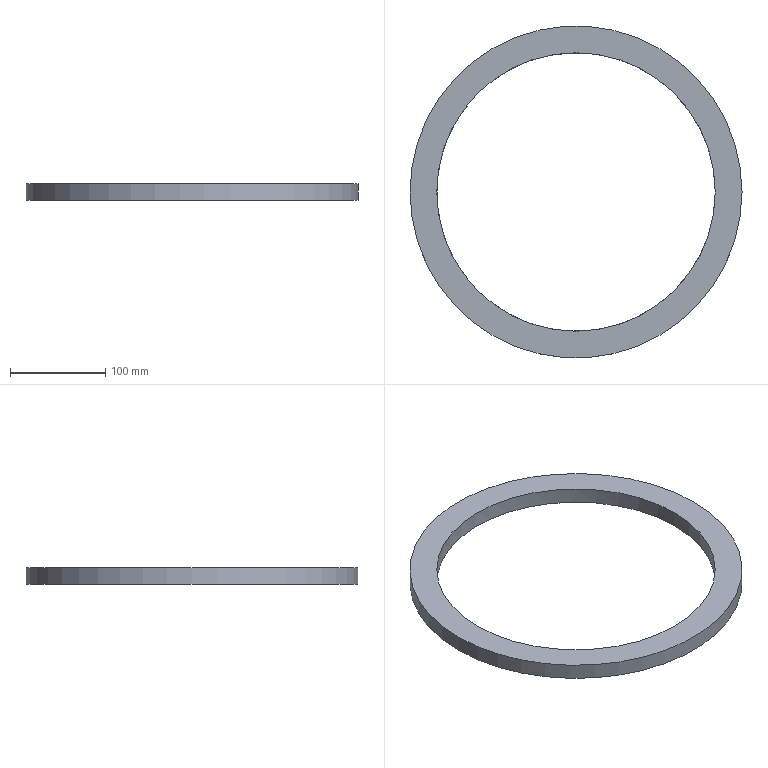Part | NX | features CYLINDER 2, DATUM_CSYS 1, Delete Body 1, LINKED_BODY 1, SCALE 1 | 1 solid | 4 faces | box 348.75 x 348.75 x 16.875 mm | volume 478061 mm3 | plane 2 | cylinder 2 | commonest cylinder face diameters 292.5 x1 348.75 x1
STEP:
#1=CARTESIAN_POINT('',(-512.832,-1724.979,-139.));
#2=VERTEX_POINT('',#1);
#3=CARTESIAN_POINT('',(-366.582,-1724.979,-139.));
#4=DIRECTION('',(0.,0.,-1.));
#5=DIRECTION('',(-1.,0.,0.));
#6=AXIS2_PLACEMENT_3D('',#3,#4,#5);
#7=CIRCLE('',#6,146.25);
#8=EDGE_CURVE('',#2,#2,#7,.T.);
#9=ORIENTED_EDGE('',*,*,#8,.T.);
#10=EDGE_LOOP('',(#9));
#11=FACE_BOUND('',#10,.T.);
#12=CARTESIAN_POINT('',(-540.957,-1724.979,-139.));
#13=VERTEX_POINT('',#12);
#14=CARTESIAN_POINT('',(-366.582,-1724.979,-139.));
#15=DIRECTION('',(0.,0.,-1.));
#16=DIRECTION('',(-1.,0.,0.));
#17=AXIS2_PLACEMENT_3D('',#14,#15,#16);
#18=CIRCLE('',#17,174.375);
#19=EDGE_CURVE('',#13,#13,#18,.T.);
#20=ORIENTED_EDGE('',*,*,#19,.F.);
#21=EDGE_LOOP('',(#20));
#22=FACE_BOUND('',#21,.T.);
#23=CARTESIAN_POINT('',(-366.582,-1724.979,-139.));
#24=DIRECTION('',(0.,0.,1.));
#25=DIRECTION('',(1.,0.,0.));
#26=AXIS2_PLACEMENT_3D('',#23,#24,#25);
#27=PLANE('',#26);
#28=ADVANCED_FACE('',(#11,#22),#27,.T.);
#29=CARTESIAN_POINT('',(-220.332,-1724.979,-155.875));
#30=VERTEX_POINT('',#29);
#31=CARTESIAN_POINT('',(-366.582,-1724.979,-155.875));
#32=DIRECTION('',(0.,0.,1.));
#33=DIRECTION('',(1.,0.,0.));
#34=AXIS2_PLACEMENT_3D('',#31,#32,#33);
#35=CIRCLE('',#34,146.25);
#36=EDGE_CURVE('',#30,#30,#35,.T.);
#37=ORIENTED_EDGE('',*,*,#36,.T.);
#38=EDGE_LOOP('',(#37));
#39=FACE_BOUND('',#38,.T.);
#40=CARTESIAN_POINT('',(-192.207,-1724.979,-155.875));
#41=VERTEX_POINT('',#40);
#42=CARTESIAN_POINT('',(-366.582,-1724.979,-155.875));
#43=DIRECTION('',(0.,0.,1.));
#44=DIRECTION('',(1.,0.,0.));
#45=AXIS2_PLACEMENT_3D('',#42,#43,#44);
#46=CIRCLE('',#45,174.375);
#47=EDGE_CURVE('',#41,#41,#46,.T.);
#48=ORIENTED_EDGE('',*,*,#47,.F.);
#49=EDGE_LOOP('',(#48));
#50=FACE_BOUND('',#49,.T.);
#51=CARTESIAN_POINT('',(-366.582,-1724.979,-155.875));
#52=DIRECTION('',(0.,0.,-1.));
#53=DIRECTION('',(-1.,0.,0.));
#54=AXIS2_PLACEMENT_3D('',#51,#52,#53);
#55=PLANE('',#54);
#56=ADVANCED_FACE('',(#39,#50),#55,.T.);
#57=ORIENTED_EDGE('',*,*,#19,.T.);
#58=EDGE_LOOP('',(#57));
#59=FACE_BOUND('',#58,.T.);
#60=ORIENTED_EDGE('',*,*,#47,.T.);
#61=EDGE_LOOP('',(#60));
#62=FACE_BOUND('',#61,.T.);
#63=CARTESIAN_POINT('',(-366.582,-1724.979,-155.875));
#64=DIRECTION('',(0.,0.,1.));
#65=DIRECTION('',(1.,0.,0.));
#66=AXIS2_PLACEMENT_3D('',#63,#64,#65);
#67=CYLINDRICAL_SURFACE('',#66,174.375);
#68=ADVANCED_FACE('',(#59,#62),#67,.T.);
#69=ORIENTED_EDGE('',*,*,#8,.F.);
#70=EDGE_LOOP('',(#69));
#71=FACE_BOUND('',#70,.T.);
#72=ORIENTED_EDGE('',*,*,#36,.F.);
#73=EDGE_LOOP('',(#72));
#74=FACE_BOUND('',#73,.T.);
#75=CARTESIAN_POINT('',(-366.582,-1724.979,-155.875));
#76=DIRECTION('',(0.,0.,1.));
#77=DIRECTION('',(1.,0.,0.));
#78=AXIS2_PLACEMENT_3D('',#75,#76,#77);
#79=CYLINDRICAL_SURFACE('',#78,146.25);
#80=ADVANCED_FACE('',(#71,#74),#79,.F.);
#81=CLOSED_SHELL('',(#28,#56,#68,#80));
#82=MANIFOLD_SOLID_BREP('',#81);
#83=(LENGTH_UNIT()NAMED_UNIT(*)SI_UNIT(.MILLI.,.METRE.));
#84=UNCERTAINTY_MEASURE_WITH_UNIT(LENGTH_MEASURE(0.00001),#83,'','');
#85=(NAMED_UNIT(*)PLANE_ANGLE_UNIT()SI_UNIT($,.RADIAN.));
#86=(NAMED_UNIT(*)SI_UNIT($,.STERADIAN.)SOLID_ANGLE_UNIT());
#87=(GEOMETRIC_REPRESENTATION_CONTEXT(3)GLOBAL_UNCERTAINTY_ASSIGNED_CONTEXT((#84))GLOBAL_UNIT_ASSIGNED_CONTEXT((#83,#85,#86))REPRESENTATION_CONTEXT('',''));
#88=ADVANCED_BREP_SHAPE_REPRESENTATION('',(#82),#87);